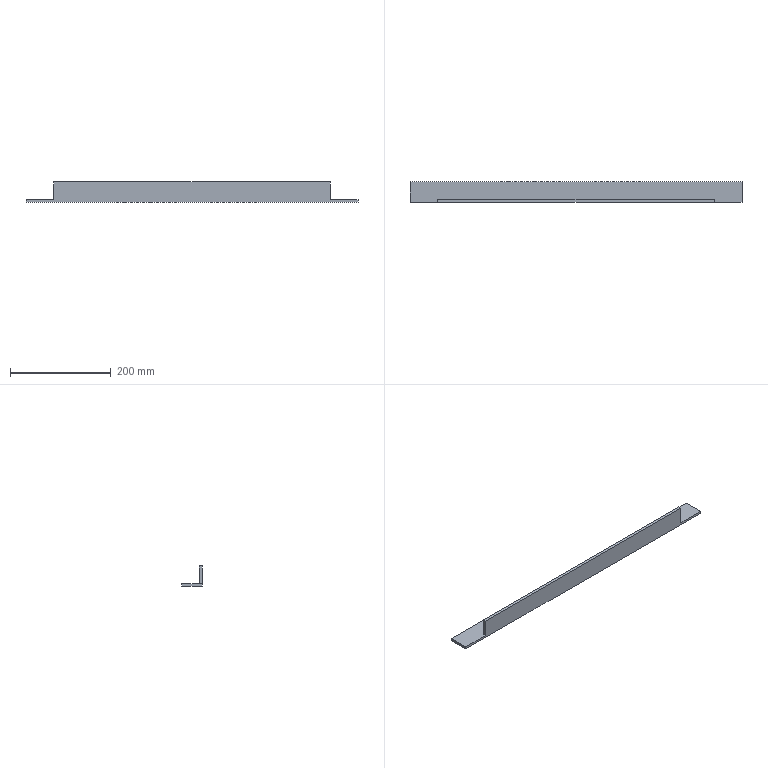Part | NX | features solid 2 | 1 solid | 10 faces | box 660 x 40 x 40 mm | volume 247500 mm3 | plane 10
STEP:
#1=CARTESIAN_POINT('',(-285.,-35.,-45.));
#2=VERTEX_POINT('',#1);
#3=CARTESIAN_POINT('',(-285.,-29.,-45.));
#4=VERTEX_POINT('',#3);
#5=CARTESIAN_POINT('',(-285.,96.,-45.));
#6=DIRECTION('',(0.,-1.,0.));
#7=VECTOR('',#6,1000.);
#8=LINE('',#5,#7);
#9=EDGE_CURVE('',#2,#4,#8,.F.);
#10=ORIENTED_EDGE('',*,*,#9,.T.);
#11=CARTESIAN_POINT('',(265.,-29.,-45.));
#12=VERTEX_POINT('',#11);
#13=CARTESIAN_POINT('',(-340.,-29.,-45.));
#14=DIRECTION('',(1.,0.,0.));
#15=VECTOR('',#14,1000.);
#16=LINE('',#13,#15);
#17=EDGE_CURVE('',#4,#12,#16,.T.);
#18=ORIENTED_EDGE('',*,*,#17,.T.);
#19=CARTESIAN_POINT('',(265.,-35.,-45.));
#20=VERTEX_POINT('',#19);
#21=CARTESIAN_POINT('',(265.,-35.,-45.));
#22=DIRECTION('',(0.,-1.,0.));
#23=VECTOR('',#22,1000.);
#24=LINE('',#21,#23);
#25=EDGE_CURVE('',#20,#12,#24,.F.);
#26=ORIENTED_EDGE('',*,*,#25,.F.);
#27=CARTESIAN_POINT('',(320.,-35.,-45.));
#28=VERTEX_POINT('',#27);
#29=CARTESIAN_POINT('',(-360.,-35.,-45.));
#30=DIRECTION('',(-1.,0.,0.));
#31=VECTOR('',#30,1000.);
#32=LINE('',#29,#31);
#33=EDGE_CURVE('',#20,#28,#32,.F.);
#34=ORIENTED_EDGE('',*,*,#33,.T.);
#35=CARTESIAN_POINT('',(320.,5.,-45.));
#36=VERTEX_POINT('',#35);
#37=CARTESIAN_POINT('',(320.,-35.,-45.));
#38=DIRECTION('',(0.,-1.,0.));
#39=VECTOR('',#38,1000.);
#40=LINE('',#37,#39);
#41=EDGE_CURVE('',#28,#36,#40,.F.);
#42=ORIENTED_EDGE('',*,*,#41,.T.);
#43=CARTESIAN_POINT('',(-340.,5.,-45.));
#44=VERTEX_POINT('',#43);
#45=CARTESIAN_POINT('',(-360.,5.,-45.));
#46=DIRECTION('',(1.,0.,0.));
#47=VECTOR('',#46,1000.);
#48=LINE('',#45,#47);
#49=EDGE_CURVE('',#44,#36,#48,.T.);
#50=ORIENTED_EDGE('',*,*,#49,.F.);
#51=CARTESIAN_POINT('',(-340.,-35.,-45.));
#52=VERTEX_POINT('',#51);
#53=CARTESIAN_POINT('',(-340.,-35.,-45.));
#54=DIRECTION('',(0.,1.,0.));
#55=VECTOR('',#54,1000.);
#56=LINE('',#53,#55);
#57=EDGE_CURVE('',#52,#44,#56,.T.);
#58=ORIENTED_EDGE('',*,*,#57,.F.);
#59=CARTESIAN_POINT('',(-360.,-35.,-45.));
#60=DIRECTION('',(-1.,0.,0.));
#61=VECTOR('',#60,1000.);
#62=LINE('',#59,#61);
#63=EDGE_CURVE('',#52,#2,#62,.F.);
#64=ORIENTED_EDGE('',*,*,#63,.T.);
#65=EDGE_LOOP('',(#10,#18,#26,#34,#42,#50,#58,#64));
#66=FACE_BOUND('',#65,.T.);
#67=CARTESIAN_POINT('',(-360.,-35.,-45.));
#68=DIRECTION('',(0.,0.,-1.));
#69=DIRECTION('',(-1.,0.,0.));
#70=AXIS2_PLACEMENT_3D('',#67,#68,#69);
#71=PLANE('',#70);
#72=ADVANCED_FACE('',(#66),#71,.F.);
#73=CARTESIAN_POINT('',(-340.,-35.,-50.));
#74=VERTEX_POINT('',#73);
#75=CARTESIAN_POINT('',(320.,-35.,-50.));
#76=VERTEX_POINT('',#75);
#77=CARTESIAN_POINT('',(-360.,-35.,-50.));
#78=DIRECTION('',(-1.,0.,0.));
#79=VECTOR('',#78,1000.);
#80=LINE('',#77,#79);
#81=EDGE_CURVE('',#74,#76,#80,.F.);
#82=ORIENTED_EDGE('',*,*,#81,.T.);
#83=CARTESIAN_POINT('',(320.,-35.,-44.));
#84=DIRECTION('',(0.,0.,-1.));
#85=VECTOR('',#84,1000.);
#86=LINE('',#83,#85);
#87=EDGE_CURVE('',#28,#76,#86,.T.);
#88=ORIENTED_EDGE('',*,*,#87,.F.);
#89=ORIENTED_EDGE('',*,*,#33,.F.);
#90=CARTESIAN_POINT('',(265.,-35.,-10.));
#91=VERTEX_POINT('',#90);
#92=CARTESIAN_POINT('',(265.,-35.,-44.));
#93=DIRECTION('',(0.,0.,-1.));
#94=VECTOR('',#93,1000.);
#95=LINE('',#92,#94);
#96=EDGE_CURVE('',#20,#91,#95,.F.);
#97=ORIENTED_EDGE('',*,*,#96,.T.);
#98=CARTESIAN_POINT('',(-285.,-35.,-10.));
#99=VERTEX_POINT('',#98);
#100=CARTESIAN_POINT('',(-340.,-35.,-10.));
#101=DIRECTION('',(1.,0.,0.));
#102=VECTOR('',#101,1000.);
#103=LINE('',#100,#102);
#104=EDGE_CURVE('',#99,#91,#103,.T.);
#105=ORIENTED_EDGE('',*,*,#104,.F.);
#106=CARTESIAN_POINT('',(-285.,-35.,-45.));
#107=DIRECTION('',(0.,0.,-1.));
#108=VECTOR('',#107,1000.);
#109=LINE('',#106,#108);
#110=EDGE_CURVE('',#2,#99,#109,.F.);
#111=ORIENTED_EDGE('',*,*,#110,.F.);
#112=ORIENTED_EDGE('',*,*,#63,.F.);
#113=CARTESIAN_POINT('',(-340.,-35.,-44.));
#114=DIRECTION('',(0.,0.,1.));
#115=VECTOR('',#114,1000.);
#116=LINE('',#113,#115);
#117=EDGE_CURVE('',#52,#74,#116,.F.);
#118=ORIENTED_EDGE('',*,*,#117,.T.);
#119=EDGE_LOOP('',(#82,#88,#89,#97,#105,#111,#112,#118));
#120=FACE_BOUND('',#119,.T.);
#121=CARTESIAN_POINT('',(-360.,-35.,-44.));
#122=DIRECTION('',(0.,-1.,0.));
#123=DIRECTION('',(1.,0.,0.));
#124=AXIS2_PLACEMENT_3D('',#121,#122,#123);
#125=PLANE('',#124);
#126=ADVANCED_FACE('',(#120),#125,.T.);
#127=ORIENTED_EDGE('',*,*,#117,.F.);
#128=ORIENTED_EDGE('',*,*,#57,.T.);
#129=CARTESIAN_POINT('',(-340.,5.,-50.));
#130=VERTEX_POINT('',#129);
#131=CARTESIAN_POINT('',(-340.,5.,-50.));
#132=DIRECTION('',(0.,0.,1.));
#133=VECTOR('',#132,1000.);
#134=LINE('',#131,#133);
#135=EDGE_CURVE('',#130,#44,#134,.T.);
#136=ORIENTED_EDGE('',*,*,#135,.F.);
#137=CARTESIAN_POINT('',(-340.,5.,-50.));
#138=DIRECTION('',(0.,-1.,0.));
#139=VECTOR('',#138,1000.);
#140=LINE('',#137,#139);
#141=EDGE_CURVE('',#130,#74,#140,.T.);
#142=ORIENTED_EDGE('',*,*,#141,.T.);
#143=EDGE_LOOP('',(#127,#128,#136,#142));
#144=FACE_BOUND('',#143,.T.);
#145=CARTESIAN_POINT('',(-340.,-35.,-44.));
#146=DIRECTION('',(1.,0.,0.));
#147=DIRECTION('',(0.,1.,0.));
#148=AXIS2_PLACEMENT_3D('',#145,#146,#147);
#149=PLANE('',#148);
#150=ADVANCED_FACE('',(#144),#149,.F.);
#151=ORIENTED_EDGE('',*,*,#41,.F.);
#152=ORIENTED_EDGE('',*,*,#87,.T.);
#153=CARTESIAN_POINT('',(320.,5.,-50.));
#154=VERTEX_POINT('',#153);
#155=CARTESIAN_POINT('',(320.,-35.,-50.));
#156=DIRECTION('',(0.,1.,0.));
#157=VECTOR('',#156,1000.);
#158=LINE('',#155,#157);
#159=EDGE_CURVE('',#154,#76,#158,.F.);
#160=ORIENTED_EDGE('',*,*,#159,.F.);
#161=CARTESIAN_POINT('',(320.,5.,-44.));
#162=DIRECTION('',(0.,0.,-1.));
#163=VECTOR('',#162,1000.);
#164=LINE('',#161,#163);
#165=EDGE_CURVE('',#154,#36,#164,.F.);
#166=ORIENTED_EDGE('',*,*,#165,.T.);
#167=EDGE_LOOP('',(#151,#152,#160,#166));
#168=FACE_BOUND('',#167,.T.);
#169=CARTESIAN_POINT('',(320.,-35.,-44.));
#170=DIRECTION('',(1.,0.,0.));
#171=DIRECTION('',(0.,1.,0.));
#172=AXIS2_PLACEMENT_3D('',#169,#170,#171);
#173=PLANE('',#172);
#174=ADVANCED_FACE('',(#168),#173,.T.);
#175=ORIENTED_EDGE('',*,*,#141,.F.);
#176=CARTESIAN_POINT('',(-360.,5.,-50.));
#177=DIRECTION('',(1.,0.,0.));
#178=VECTOR('',#177,1000.);
#179=LINE('',#176,#178);
#180=EDGE_CURVE('',#130,#154,#179,.T.);
#181=ORIENTED_EDGE('',*,*,#180,.T.);
#182=ORIENTED_EDGE('',*,*,#159,.T.);
#183=ORIENTED_EDGE('',*,*,#81,.F.);
#184=EDGE_LOOP('',(#175,#181,#182,#183));
#185=FACE_BOUND('',#184,.T.);
#186=CARTESIAN_POINT('',(-360.,5.,-50.));
#187=DIRECTION('',(0.,0.,1.));
#188=DIRECTION('',(1.,0.,0.));
#189=AXIS2_PLACEMENT_3D('',#186,#187,#188);
#190=PLANE('',#189);
#191=ADVANCED_FACE('',(#185),#190,.F.);
#192=ORIENTED_EDGE('',*,*,#135,.T.);
#193=ORIENTED_EDGE('',*,*,#49,.T.);
#194=ORIENTED_EDGE('',*,*,#165,.F.);
#195=ORIENTED_EDGE('',*,*,#180,.F.);
#196=EDGE_LOOP('',(#192,#193,#194,#195));
#197=FACE_BOUND('',#196,.T.);
#198=CARTESIAN_POINT('',(-360.,5.,-50.));
#199=DIRECTION('',(0.,1.,0.));
#200=DIRECTION('',(1.,0.,0.));
#201=AXIS2_PLACEMENT_3D('',#198,#199,#200);
#202=PLANE('',#201);
#203=ADVANCED_FACE('',(#197),#202,.T.);
#204=ORIENTED_EDGE('',*,*,#110,.T.);
#205=CARTESIAN_POINT('',(-285.,-29.,-10.));
#206=VERTEX_POINT('',#205);
#207=CARTESIAN_POINT('',(-285.,96.,-10.));
#208=DIRECTION('',(0.,-1.,0.));
#209=VECTOR('',#208,1000.);
#210=LINE('',#207,#209);
#211=EDGE_CURVE('',#99,#206,#210,.F.);
#212=ORIENTED_EDGE('',*,*,#211,.T.);
#213=CARTESIAN_POINT('',(-285.,-29.,-12.));
#214=DIRECTION('',(0.,0.,1.));
#215=VECTOR('',#214,1000.);
#216=LINE('',#213,#215);
#217=EDGE_CURVE('',#4,#206,#216,.T.);
#218=ORIENTED_EDGE('',*,*,#217,.F.);
#219=ORIENTED_EDGE('',*,*,#9,.F.);
#220=EDGE_LOOP('',(#204,#212,#218,#219));
#221=FACE_BOUND('',#220,.T.);
#222=CARTESIAN_POINT('',(-285.,96.,-12.));
#223=DIRECTION('',(1.,0.,0.));
#224=DIRECTION('',(0.,0.,-1.));
#225=AXIS2_PLACEMENT_3D('',#222,#223,#224);
#226=PLANE('',#225);
#227=ADVANCED_FACE('',(#221),#226,.F.);
#228=ORIENTED_EDGE('',*,*,#217,.T.);
#229=CARTESIAN_POINT('',(265.,-29.,-10.));
#230=VERTEX_POINT('',#229);
#231=CARTESIAN_POINT('',(-340.,-29.,-10.));
#232=DIRECTION('',(-1.,0.,0.));
#233=VECTOR('',#232,1000.);
#234=LINE('',#231,#233);
#235=EDGE_CURVE('',#206,#230,#234,.F.);
#236=ORIENTED_EDGE('',*,*,#235,.T.);
#237=CARTESIAN_POINT('',(265.,-29.,-45.));
#238=DIRECTION('',(0.,0.,1.));
#239=VECTOR('',#238,1000.);
#240=LINE('',#237,#239);
#241=EDGE_CURVE('',#12,#230,#240,.T.);
#242=ORIENTED_EDGE('',*,*,#241,.F.);
#243=ORIENTED_EDGE('',*,*,#17,.F.);
#244=EDGE_LOOP('',(#228,#236,#242,#243));
#245=FACE_BOUND('',#244,.T.);
#246=CARTESIAN_POINT('',(-340.,-29.,-45.));
#247=DIRECTION('',(0.,-1.,0.));
#248=DIRECTION('',(1.,0.,0.));
#249=AXIS2_PLACEMENT_3D('',#246,#247,#248);
#250=PLANE('',#249);
#251=ADVANCED_FACE('',(#245),#250,.F.);
#252=ORIENTED_EDGE('',*,*,#25,.T.);
#253=ORIENTED_EDGE('',*,*,#241,.T.);
#254=CARTESIAN_POINT('',(265.,-35.,-10.));
#255=DIRECTION('',(0.,-1.,0.));
#256=VECTOR('',#255,1000.);
#257=LINE('',#254,#256);
#258=EDGE_CURVE('',#91,#230,#257,.F.);
#259=ORIENTED_EDGE('',*,*,#258,.F.);
#260=ORIENTED_EDGE('',*,*,#96,.F.);
#261=EDGE_LOOP('',(#252,#253,#259,#260));
#262=FACE_BOUND('',#261,.T.);
#263=CARTESIAN_POINT('',(265.,361.,-44.));
#264=DIRECTION('',(-1.,0.,0.));
#265=DIRECTION('',(0.,0.,1.));
#266=AXIS2_PLACEMENT_3D('',#263,#264,#265);
#267=PLANE('',#266);
#268=ADVANCED_FACE('',(#262),#267,.F.);
#269=ORIENTED_EDGE('',*,*,#235,.F.);
#270=ORIENTED_EDGE('',*,*,#211,.F.);
#271=ORIENTED_EDGE('',*,*,#104,.T.);
#272=ORIENTED_EDGE('',*,*,#258,.T.);
#273=EDGE_LOOP('',(#269,#270,#271,#272));
#274=FACE_BOUND('',#273,.T.);
#275=CARTESIAN_POINT('',(-340.,-35.,-10.));
#276=DIRECTION('',(0.,0.,-1.));
#277=DIRECTION('',(-1.,0.,0.));
#278=AXIS2_PLACEMENT_3D('',#275,#276,#277);
#279=PLANE('',#278);
#280=ADVANCED_FACE('',(#274),#279,.F.);
#281=CLOSED_SHELL('',(#72,#126,#150,#174,#191,#203,#227,#251,#268,#280));
#282=MANIFOLD_SOLID_BREP('',#281);
#283=(LENGTH_UNIT()NAMED_UNIT(*)SI_UNIT(.MILLI.,.METRE.));
#284=UNCERTAINTY_MEASURE_WITH_UNIT(LENGTH_MEASURE(0.00001),#283,'','');
#285=(NAMED_UNIT(*)PLANE_ANGLE_UNIT()SI_UNIT($,.RADIAN.));
#286=(NAMED_UNIT(*)SI_UNIT($,.STERADIAN.)SOLID_ANGLE_UNIT());
#287=(GEOMETRIC_REPRESENTATION_CONTEXT(3)GLOBAL_UNCERTAINTY_ASSIGNED_CONTEXT((#284))GLOBAL_UNIT_ASSIGNED_CONTEXT((#283,#285,#286))REPRESENTATION_CONTEXT('',''));
#288=ADVANCED_BREP_SHAPE_REPRESENTATION('',(#282),#287);